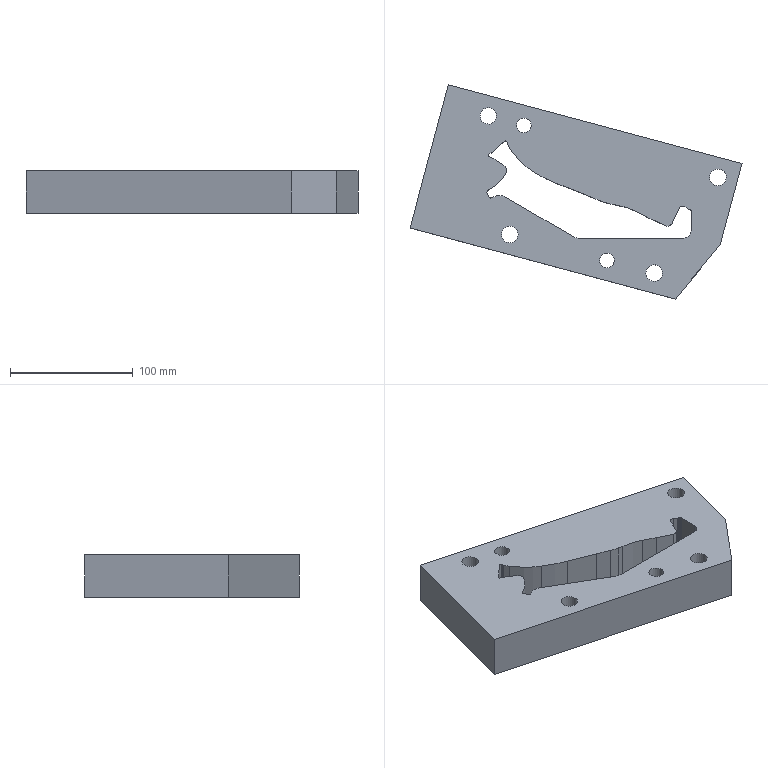Part | NX | features 7 2 | 1 solid | 85 faces | box 270.867 x 174.868 x 35 mm | volume 804507 mm3 | plane 37 | cylinder 32 | spline 14 | cone 2 | commonest cylinder face diameters 2 x8 20 x5 13.5 x4 5.199 x2 10 x2 12.001 x2